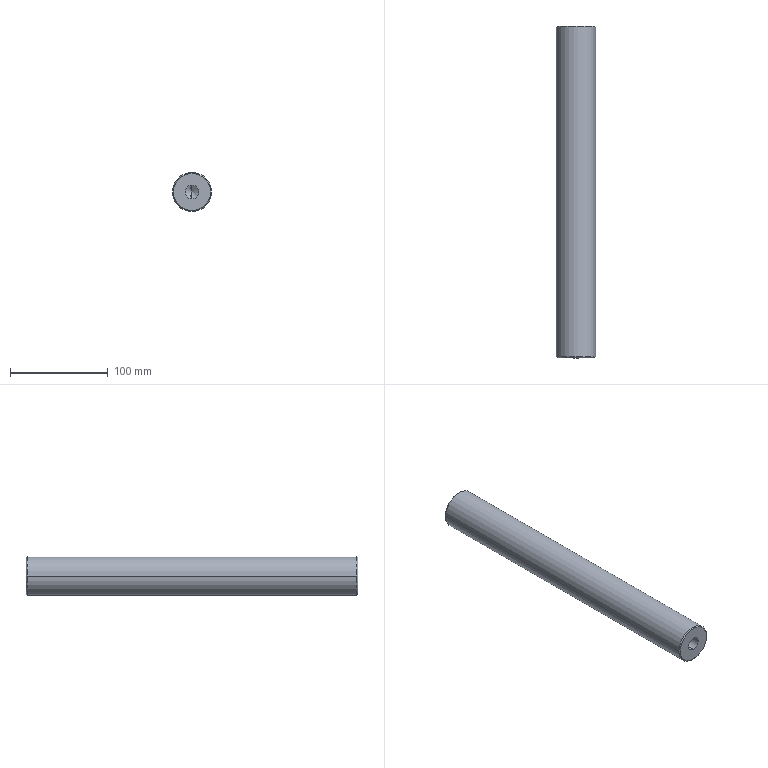Part | SolidWorks | features BaseBody 1 | 1 solid | 16 faces | box 40 x 340 x 40 mm | volume 415002 mm3 | cone 8 | cylinder 6 | plane 2 | commonest cylinder face diameters 14 x4 40 x2
STEP:
#1=CARTESIAN_POINT('',(0.,-132.,7.));
#2=VERTEX_POINT('',#1);
#3=CARTESIAN_POINT('',(0.,-132.,-7.));
#4=VERTEX_POINT('',#3);
#5=CARTESIAN_POINT('',(0.,-132.,0.));
#6=DIRECTION('',(0.,-1.,0.));
#7=DIRECTION('',(0.,0.,-1.));
#8=AXIS2_PLACEMENT_3D('',#5,#6,#7);
#9=CIRCLE('',#8,7.);
#10=EDGE_CURVE('',#2,#4,#9,.T.);
#11=ORIENTED_EDGE('',*,*,#10,.F.);
#12=CARTESIAN_POINT('',(0.,-170.,7.));
#13=VERTEX_POINT('',#12);
#14=CARTESIAN_POINT('',(0.,-170.,7.));
#15=DIRECTION('',(0.,-1.,0.));
#16=VECTOR('',#15,1000.);
#17=LINE('',#14,#16);
#18=EDGE_CURVE('',#2,#13,#17,.T.);
#19=ORIENTED_EDGE('',*,*,#18,.T.);
#20=CARTESIAN_POINT('',(0.,-170.,-7.));
#21=VERTEX_POINT('',#20);
#22=CARTESIAN_POINT('',(0.,-170.,0.));
#23=DIRECTION('',(0.,-1.,0.));
#24=DIRECTION('',(0.,0.,-1.));
#25=AXIS2_PLACEMENT_3D('',#22,#23,#24);
#26=CIRCLE('',#25,7.);
#27=EDGE_CURVE('',#13,#21,#26,.T.);
#28=ORIENTED_EDGE('',*,*,#27,.T.);
#29=CARTESIAN_POINT('',(0.,-170.,-7.));
#30=DIRECTION('',(0.,-1.,0.));
#31=VECTOR('',#30,1000.);
#32=LINE('',#29,#31);
#33=EDGE_CURVE('',#4,#21,#32,.T.);
#34=ORIENTED_EDGE('',*,*,#33,.F.);
#35=EDGE_LOOP('',(#11,#19,#28,#34));
#36=FACE_OUTER_BOUND('',#35,.T.);
#37=CARTESIAN_POINT('',(0.,-170.,0.));
#38=DIRECTION('',(0.,-1.,0.));
#39=DIRECTION('',(0.,0.,-1.));
#40=AXIS2_PLACEMENT_3D('',#37,#38,#39);
#41=CYLINDRICAL_SURFACE('',#40,7.);
#42=ADVANCED_FACE('',(#36),#41,.F.);
#43=CARTESIAN_POINT('',(0.,-127.794,0.));
#44=VERTEX_POINT('',#43);
#45=CARTESIAN_POINT('',(0.,-132.,-7.));
#46=DIRECTION('',(0.,-0.515,-0.8572));
#47=VECTOR('',#46,1000.);
#48=LINE('',#45,#47);
#49=EDGE_CURVE('',#44,#4,#48,.T.);
#50=ORIENTED_EDGE('',*,*,#49,.F.);
#51=CARTESIAN_POINT('',(0.,-132.,7.));
#52=DIRECTION('',(0.,-0.515,0.8572));
#53=VECTOR('',#52,1000.);
#54=LINE('',#51,#53);
#55=EDGE_CURVE('',#44,#2,#54,.T.);
#56=ORIENTED_EDGE('',*,*,#55,.T.);
#57=ORIENTED_EDGE('',*,*,#10,.T.);
#58=EDGE_LOOP('',(#50,#56,#57));
#59=FACE_OUTER_BOUND('',#58,.T.);
#60=CARTESIAN_POINT('',(0.,-132.,0.));
#61=DIRECTION('',(0.,-1.,0.));
#62=DIRECTION('',(0.,0.,-1.));
#63=AXIS2_PLACEMENT_3D('',#60,#61,#62);
#64=CONICAL_SURFACE('',#63,7.,1.03);
#65=ADVANCED_FACE('',(#59),#64,.F.);
#66=CARTESIAN_POINT('',(0.,132.,-7.));
#67=VERTEX_POINT('',#66);
#68=CARTESIAN_POINT('',(0.,132.,7.));
#69=VERTEX_POINT('',#68);
#70=CARTESIAN_POINT('',(0.,132.,0.));
#71=DIRECTION('',(0.,1.,0.));
#72=DIRECTION('',(0.,0.,1.));
#73=AXIS2_PLACEMENT_3D('',#70,#71,#72);
#74=CIRCLE('',#73,7.);
#75=EDGE_CURVE('',#67,#69,#74,.T.);
#76=ORIENTED_EDGE('',*,*,#75,.F.);
#77=CARTESIAN_POINT('',(0.,170.,-7.));
#78=VERTEX_POINT('',#77);
#79=CARTESIAN_POINT('',(0.,170.,-7.));
#80=DIRECTION('',(0.,1.,0.));
#81=VECTOR('',#80,1000.);
#82=LINE('',#79,#81);
#83=EDGE_CURVE('',#67,#78,#82,.T.);
#84=ORIENTED_EDGE('',*,*,#83,.T.);
#85=CARTESIAN_POINT('',(0.,170.,7.));
#86=VERTEX_POINT('',#85);
#87=CARTESIAN_POINT('',(0.,170.,0.));
#88=DIRECTION('',(0.,1.,0.));
#89=DIRECTION('',(0.,0.,1.));
#90=AXIS2_PLACEMENT_3D('',#87,#88,#89);
#91=CIRCLE('',#90,7.);
#92=EDGE_CURVE('',#78,#86,#91,.T.);
#93=ORIENTED_EDGE('',*,*,#92,.T.);
#94=CARTESIAN_POINT('',(0.,170.,7.));
#95=DIRECTION('',(0.,1.,0.));
#96=VECTOR('',#95,1000.);
#97=LINE('',#94,#96);
#98=EDGE_CURVE('',#69,#86,#97,.T.);
#99=ORIENTED_EDGE('',*,*,#98,.F.);
#100=EDGE_LOOP('',(#76,#84,#93,#99));
#101=FACE_OUTER_BOUND('',#100,.T.);
#102=CARTESIAN_POINT('',(0.,170.,0.));
#103=DIRECTION('',(0.,1.,0.));
#104=DIRECTION('',(0.,0.,1.));
#105=AXIS2_PLACEMENT_3D('',#102,#103,#104);
#106=CYLINDRICAL_SURFACE('',#105,7.);
#107=ADVANCED_FACE('',(#101),#106,.F.);
#108=CARTESIAN_POINT('',(0.,127.794,0.));
#109=VERTEX_POINT('',#108);
#110=CARTESIAN_POINT('',(0.,132.,7.));
#111=DIRECTION('',(0.,0.515,0.8572));
#112=VECTOR('',#111,1000.);
#113=LINE('',#110,#112);
#114=EDGE_CURVE('',#109,#69,#113,.T.);
#115=ORIENTED_EDGE('',*,*,#114,.F.);
#116=CARTESIAN_POINT('',(0.,132.,-7.));
#117=DIRECTION('',(0.,0.515,-0.8572));
#118=VECTOR('',#117,1000.);
#119=LINE('',#116,#118);
#120=EDGE_CURVE('',#109,#67,#119,.T.);
#121=ORIENTED_EDGE('',*,*,#120,.T.);
#122=ORIENTED_EDGE('',*,*,#75,.T.);
#123=EDGE_LOOP('',(#115,#121,#122));
#124=FACE_OUTER_BOUND('',#123,.T.);
#125=CARTESIAN_POINT('',(0.,132.,0.));
#126=DIRECTION('',(0.,1.,0.));
#127=DIRECTION('',(0.,0.,1.));
#128=AXIS2_PLACEMENT_3D('',#125,#126,#127);
#129=CONICAL_SURFACE('',#128,7.,1.03);
#130=ADVANCED_FACE('',(#124),#129,.F.);
#131=CARTESIAN_POINT('',(-19.,170.,0.));
#132=VERTEX_POINT('',#131);
#133=CARTESIAN_POINT('',(19.,170.,0.));
#134=VERTEX_POINT('',#133);
#135=CARTESIAN_POINT('',(0.,170.,0.));
#136=DIRECTION('',(0.,1.,0.));
#137=DIRECTION('',(-1.,0.,0.));
#138=AXIS2_PLACEMENT_3D('',#135,#136,#137);
#139=CIRCLE('',#138,19.);
#140=EDGE_CURVE('',#132,#134,#139,.T.);
#141=ORIENTED_EDGE('',*,*,#140,.F.);
#142=CARTESIAN_POINT('',(-20.,169.,0.));
#143=VERTEX_POINT('',#142);
#144=CARTESIAN_POINT('',(-20.,169.,0.));
#145=DIRECTION('',(-0.7071,-0.7071,0.));
#146=VECTOR('',#145,1000.);
#147=LINE('',#144,#146);
#148=EDGE_CURVE('',#132,#143,#147,.T.);
#149=ORIENTED_EDGE('',*,*,#148,.T.);
#150=CARTESIAN_POINT('',(20.,169.,0.));
#151=VERTEX_POINT('',#150);
#152=CARTESIAN_POINT('',(0.,169.,0.));
#153=DIRECTION('',(0.,1.,0.));
#154=DIRECTION('',(-1.,0.,0.));
#155=AXIS2_PLACEMENT_3D('',#152,#153,#154);
#156=CIRCLE('',#155,20.);
#157=EDGE_CURVE('',#143,#151,#156,.T.);
#158=ORIENTED_EDGE('',*,*,#157,.T.);
#159=CARTESIAN_POINT('',(20.,169.,0.));
#160=DIRECTION('',(0.7071,-0.7071,0.));
#161=VECTOR('',#160,1000.);
#162=LINE('',#159,#161);
#163=EDGE_CURVE('',#134,#151,#162,.T.);
#164=ORIENTED_EDGE('',*,*,#163,.F.);
#165=EDGE_LOOP('',(#141,#149,#158,#164));
#166=FACE_OUTER_BOUND('',#165,.T.);
#167=CARTESIAN_POINT('',(0.,169.,0.));
#168=DIRECTION('',(0.,-1.,0.));
#169=DIRECTION('',(1.,0.,0.));
#170=AXIS2_PLACEMENT_3D('',#167,#168,#169);
#171=CONICAL_SURFACE('',#170,20.,0.7854);
#172=ADVANCED_FACE('',(#166),#171,.T.);
#173=CARTESIAN_POINT('',(-20.,-169.,0.));
#174=VERTEX_POINT('',#173);
#175=CARTESIAN_POINT('',(20.,-169.,0.));
#176=VERTEX_POINT('',#175);
#177=CARTESIAN_POINT('',(0.,-169.,0.));
#178=DIRECTION('',(0.,1.,0.));
#179=DIRECTION('',(-1.,0.,0.));
#180=AXIS2_PLACEMENT_3D('',#177,#178,#179);
#181=CIRCLE('',#180,20.);
#182=EDGE_CURVE('',#174,#176,#181,.T.);
#183=ORIENTED_EDGE('',*,*,#182,.T.);
#184=CARTESIAN_POINT('',(20.,170.,0.));
#185=DIRECTION('',(0.,1.,0.));
#186=VECTOR('',#185,1000.);
#187=LINE('',#184,#186);
#188=EDGE_CURVE('',#176,#151,#187,.T.);
#189=ORIENTED_EDGE('',*,*,#188,.T.);
#190=ORIENTED_EDGE('',*,*,#157,.F.);
#191=CARTESIAN_POINT('',(-20.,170.,0.));
#192=DIRECTION('',(0.,1.,0.));
#193=VECTOR('',#192,1000.);
#194=LINE('',#191,#193);
#195=EDGE_CURVE('',#174,#143,#194,.T.);
#196=ORIENTED_EDGE('',*,*,#195,.F.);
#197=EDGE_LOOP('',(#183,#189,#190,#196));
#198=FACE_OUTER_BOUND('',#197,.T.);
#199=CARTESIAN_POINT('',(0.,170.,0.));
#200=DIRECTION('',(0.,1.,0.));
#201=DIRECTION('',(-1.,0.,0.));
#202=AXIS2_PLACEMENT_3D('',#199,#200,#201);
#203=CYLINDRICAL_SURFACE('',#202,20.);
#204=ADVANCED_FACE('',(#198),#203,.T.);
#205=CARTESIAN_POINT('',(-19.,-170.,0.));
#206=VERTEX_POINT('',#205);
#207=CARTESIAN_POINT('',(19.,-170.,0.));
#208=VERTEX_POINT('',#207);
#209=CARTESIAN_POINT('',(0.,-170.,0.));
#210=DIRECTION('',(0.,1.,0.));
#211=DIRECTION('',(-1.,0.,0.));
#212=AXIS2_PLACEMENT_3D('',#209,#210,#211);
#213=CIRCLE('',#212,19.);
#214=EDGE_CURVE('',#206,#208,#213,.T.);
#215=ORIENTED_EDGE('',*,*,#214,.T.);
#216=CARTESIAN_POINT('',(19.,-170.,0.));
#217=DIRECTION('',(0.7071,0.7071,0.));
#218=VECTOR('',#217,1000.);
#219=LINE('',#216,#218);
#220=EDGE_CURVE('',#208,#176,#219,.T.);
#221=ORIENTED_EDGE('',*,*,#220,.T.);
#222=ORIENTED_EDGE('',*,*,#182,.F.);
#223=CARTESIAN_POINT('',(-19.,-170.,0.));
#224=DIRECTION('',(-0.7071,0.7071,0.));
#225=VECTOR('',#224,1000.);
#226=LINE('',#223,#225);
#227=EDGE_CURVE('',#206,#174,#226,.T.);
#228=ORIENTED_EDGE('',*,*,#227,.F.);
#229=EDGE_LOOP('',(#215,#221,#222,#228));
#230=FACE_OUTER_BOUND('',#229,.T.);
#231=CARTESIAN_POINT('',(0.,-170.,0.));
#232=DIRECTION('',(0.,1.,0.));
#233=DIRECTION('',(-1.,0.,0.));
#234=AXIS2_PLACEMENT_3D('',#231,#232,#233);
#235=CONICAL_SURFACE('',#234,19.,0.7854);
#236=ADVANCED_FACE('',(#230),#235,.T.);
#237=CARTESIAN_POINT('',(0.,-170.,0.));
#238=DIRECTION('',(0.,-1.,0.));
#239=DIRECTION('',(0.,0.,-1.));
#240=AXIS2_PLACEMENT_3D('',#237,#238,#239);
#241=CIRCLE('',#240,7.);
#242=EDGE_CURVE('',#21,#13,#241,.T.);
#243=ORIENTED_EDGE('',*,*,#242,.F.);
#244=ORIENTED_EDGE('',*,*,#27,.F.);
#245=EDGE_LOOP('',(#243,#244));
#246=FACE_BOUND('',#245,.T.);
#247=ORIENTED_EDGE('',*,*,#214,.F.);
#248=CARTESIAN_POINT('',(0.,-170.,0.));
#249=DIRECTION('',(0.,1.,0.));
#250=DIRECTION('',(-1.,0.,0.));
#251=AXIS2_PLACEMENT_3D('',#248,#249,#250);
#252=CIRCLE('',#251,19.);
#253=EDGE_CURVE('',#208,#206,#252,.T.);
#254=ORIENTED_EDGE('',*,*,#253,.F.);
#255=EDGE_LOOP('',(#247,#254));
#256=FACE_OUTER_BOUND('',#255,.T.);
#257=CARTESIAN_POINT('',(0.,-170.,0.));
#258=DIRECTION('',(0.,1.,0.));
#259=DIRECTION('',(-1.,0.,0.));
#260=AXIS2_PLACEMENT_3D('',#257,#258,#259);
#261=PLANE('',#260);
#262=ADVANCED_FACE('',(#246,#256),#261,.F.);
#263=ORIENTED_EDGE('',*,*,#220,.F.);
#264=ORIENTED_EDGE('',*,*,#253,.T.);
#265=ORIENTED_EDGE('',*,*,#227,.T.);
#266=CARTESIAN_POINT('',(0.,-169.,0.));
#267=DIRECTION('',(0.,1.,0.));
#268=DIRECTION('',(-1.,0.,0.));
#269=AXIS2_PLACEMENT_3D('',#266,#267,#268);
#270=CIRCLE('',#269,20.);
#271=EDGE_CURVE('',#176,#174,#270,.T.);
#272=ORIENTED_EDGE('',*,*,#271,.F.);
#273=EDGE_LOOP('',(#263,#264,#265,#272));
#274=FACE_OUTER_BOUND('',#273,.T.);
#275=CARTESIAN_POINT('',(0.,-170.,0.));
#276=DIRECTION('',(0.,1.,0.));
#277=DIRECTION('',(-1.,0.,0.));
#278=AXIS2_PLACEMENT_3D('',#275,#276,#277);
#279=CONICAL_SURFACE('',#278,19.,0.7854);
#280=ADVANCED_FACE('',(#274),#279,.T.);
#281=ORIENTED_EDGE('',*,*,#188,.F.);
#282=ORIENTED_EDGE('',*,*,#271,.T.);
#283=ORIENTED_EDGE('',*,*,#195,.T.);
#284=CARTESIAN_POINT('',(0.,169.,0.));
#285=DIRECTION('',(0.,1.,0.));
#286=DIRECTION('',(-1.,0.,0.));
#287=AXIS2_PLACEMENT_3D('',#284,#285,#286);
#288=CIRCLE('',#287,20.);
#289=EDGE_CURVE('',#151,#143,#288,.T.);
#290=ORIENTED_EDGE('',*,*,#289,.F.);
#291=EDGE_LOOP('',(#281,#282,#283,#290));
#292=FACE_OUTER_BOUND('',#291,.T.);
#293=CARTESIAN_POINT('',(0.,170.,0.));
#294=DIRECTION('',(0.,1.,0.));
#295=DIRECTION('',(-1.,0.,0.));
#296=AXIS2_PLACEMENT_3D('',#293,#294,#295);
#297=CYLINDRICAL_SURFACE('',#296,20.);
#298=ADVANCED_FACE('',(#292),#297,.T.);
#299=ORIENTED_EDGE('',*,*,#148,.F.);
#300=CARTESIAN_POINT('',(0.,170.,0.));
#301=DIRECTION('',(0.,1.,0.));
#302=DIRECTION('',(-1.,0.,0.));
#303=AXIS2_PLACEMENT_3D('',#300,#301,#302);
#304=CIRCLE('',#303,19.);
#305=EDGE_CURVE('',#134,#132,#304,.T.);
#306=ORIENTED_EDGE('',*,*,#305,.F.);
#307=ORIENTED_EDGE('',*,*,#163,.T.);
#308=ORIENTED_EDGE('',*,*,#289,.T.);
#309=EDGE_LOOP('',(#299,#306,#307,#308));
#310=FACE_OUTER_BOUND('',#309,.T.);
#311=CARTESIAN_POINT('',(0.,169.,0.));
#312=DIRECTION('',(0.,-1.,0.));
#313=DIRECTION('',(1.,0.,0.));
#314=AXIS2_PLACEMENT_3D('',#311,#312,#313);
#315=CONICAL_SURFACE('',#314,20.,0.7854);
#316=ADVANCED_FACE('',(#310),#315,.T.);
#317=CARTESIAN_POINT('',(0.,170.,0.));
#318=DIRECTION('',(0.,1.,0.));
#319=DIRECTION('',(0.,0.,1.));
#320=AXIS2_PLACEMENT_3D('',#317,#318,#319);
#321=CIRCLE('',#320,7.);
#322=EDGE_CURVE('',#86,#78,#321,.T.);
#323=ORIENTED_EDGE('',*,*,#322,.F.);
#324=ORIENTED_EDGE('',*,*,#92,.F.);
#325=EDGE_LOOP('',(#323,#324));
#326=FACE_BOUND('',#325,.T.);
#327=ORIENTED_EDGE('',*,*,#305,.T.);
#328=ORIENTED_EDGE('',*,*,#140,.T.);
#329=EDGE_LOOP('',(#327,#328));
#330=FACE_OUTER_BOUND('',#329,.T.);
#331=CARTESIAN_POINT('',(0.,170.,0.));
#332=DIRECTION('',(0.,-1.,0.));
#333=DIRECTION('',(1.,0.,0.));
#334=AXIS2_PLACEMENT_3D('',#331,#332,#333);
#335=PLANE('',#334);
#336=ADVANCED_FACE('',(#326,#330),#335,.F.);
#337=ORIENTED_EDGE('',*,*,#120,.F.);
#338=ORIENTED_EDGE('',*,*,#114,.T.);
#339=CARTESIAN_POINT('',(0.,132.,0.));
#340=DIRECTION('',(0.,1.,0.));
#341=DIRECTION('',(0.,0.,1.));
#342=AXIS2_PLACEMENT_3D('',#339,#340,#341);
#343=CIRCLE('',#342,7.);
#344=EDGE_CURVE('',#69,#67,#343,.T.);
#345=ORIENTED_EDGE('',*,*,#344,.T.);
#346=EDGE_LOOP('',(#337,#338,#345));
#347=FACE_OUTER_BOUND('',#346,.T.);
#348=CARTESIAN_POINT('',(0.,132.,0.));
#349=DIRECTION('',(0.,1.,0.));
#350=DIRECTION('',(0.,0.,1.));
#351=AXIS2_PLACEMENT_3D('',#348,#349,#350);
#352=CONICAL_SURFACE('',#351,7.,1.03);
#353=ADVANCED_FACE('',(#347),#352,.F.);
#354=ORIENTED_EDGE('',*,*,#83,.F.);
#355=ORIENTED_EDGE('',*,*,#344,.F.);
#356=ORIENTED_EDGE('',*,*,#98,.T.);
#357=ORIENTED_EDGE('',*,*,#322,.T.);
#358=EDGE_LOOP('',(#354,#355,#356,#357));
#359=FACE_OUTER_BOUND('',#358,.T.);
#360=CARTESIAN_POINT('',(0.,170.,0.));
#361=DIRECTION('',(0.,1.,0.));
#362=DIRECTION('',(0.,0.,1.));
#363=AXIS2_PLACEMENT_3D('',#360,#361,#362);
#364=CYLINDRICAL_SURFACE('',#363,7.);
#365=ADVANCED_FACE('',(#359),#364,.F.);
#366=ORIENTED_EDGE('',*,*,#55,.F.);
#367=ORIENTED_EDGE('',*,*,#49,.T.);
#368=CARTESIAN_POINT('',(0.,-132.,0.));
#369=DIRECTION('',(0.,-1.,0.));
#370=DIRECTION('',(0.,0.,-1.));
#371=AXIS2_PLACEMENT_3D('',#368,#369,#370);
#372=CIRCLE('',#371,7.);
#373=EDGE_CURVE('',#4,#2,#372,.T.);
#374=ORIENTED_EDGE('',*,*,#373,.T.);
#375=EDGE_LOOP('',(#366,#367,#374));
#376=FACE_OUTER_BOUND('',#375,.T.);
#377=CARTESIAN_POINT('',(0.,-132.,0.));
#378=DIRECTION('',(0.,-1.,0.));
#379=DIRECTION('',(0.,0.,-1.));
#380=AXIS2_PLACEMENT_3D('',#377,#378,#379);
#381=CONICAL_SURFACE('',#380,7.,1.03);
#382=ADVANCED_FACE('',(#376),#381,.F.);
#383=ORIENTED_EDGE('',*,*,#18,.F.);
#384=ORIENTED_EDGE('',*,*,#373,.F.);
#385=ORIENTED_EDGE('',*,*,#33,.T.);
#386=ORIENTED_EDGE('',*,*,#242,.T.);
#387=EDGE_LOOP('',(#383,#384,#385,#386));
#388=FACE_OUTER_BOUND('',#387,.T.);
#389=CARTESIAN_POINT('',(0.,-170.,0.));
#390=DIRECTION('',(0.,-1.,0.));
#391=DIRECTION('',(0.,0.,-1.));
#392=AXIS2_PLACEMENT_3D('',#389,#390,#391);
#393=CYLINDRICAL_SURFACE('',#392,7.);
#394=ADVANCED_FACE('',(#388),#393,.F.);
#395=CLOSED_SHELL('',(#42,#65,#107,#130,#172,#204,#236,#262,#280,#298,#316,#336,#353,#365,#382,#394));
#396=MANIFOLD_SOLID_BREP('',#395);
#397=CARTESIAN_POINT('',(0.,0.,0.));
#398=DIRECTION('',(0.,0.,1.));
#399=DIRECTION('',(1.,0.,0.));
#400=AXIS2_PLACEMENT_3D('',#397,#398,#399);
#401=(LENGTH_UNIT()NAMED_UNIT(*)SI_UNIT(.MILLI.,.METRE.));
#402=UNCERTAINTY_MEASURE_WITH_UNIT(LENGTH_MEASURE(0.00001),#401,'','');
#403=(NAMED_UNIT(*)PLANE_ANGLE_UNIT()SI_UNIT($,.RADIAN.));
#404=(NAMED_UNIT(*)SI_UNIT($,.STERADIAN.)SOLID_ANGLE_UNIT());
#405=(GEOMETRIC_REPRESENTATION_CONTEXT(3)GLOBAL_UNCERTAINTY_ASSIGNED_CONTEXT((#402))GLOBAL_UNIT_ASSIGNED_CONTEXT((#401,#403,#404))REPRESENTATION_CONTEXT('',''));
#406=ADVANCED_BREP_SHAPE_REPRESENTATION('',(#396,#400),#405);